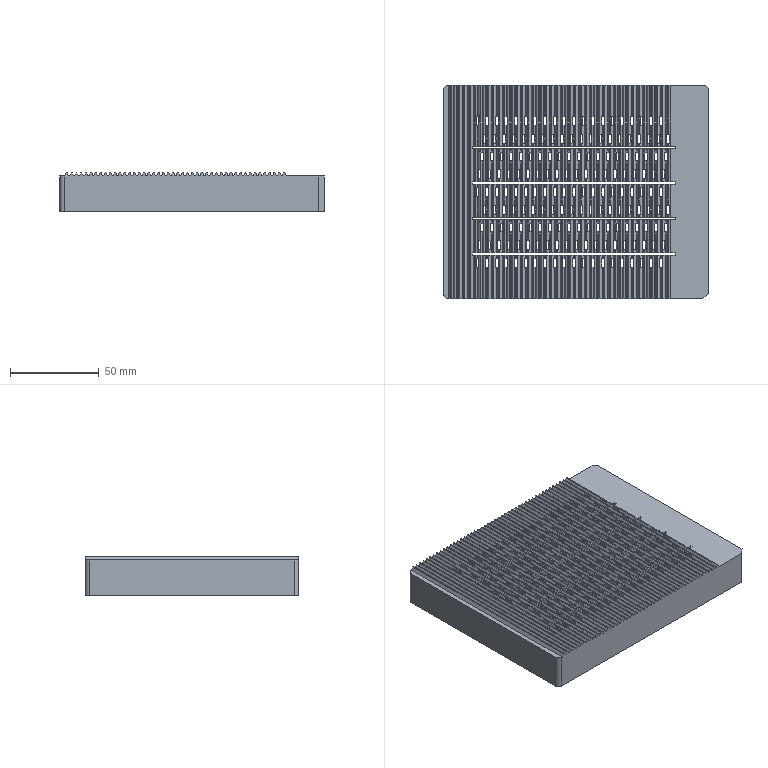Part | STEP file | 1 solid | 1774 faces | box 149 x 120 x 21.74 mm | volume 329380 mm3 | plane 1164 | cylinder 602 | cone 8 | commonest cylinder face diameters 0.8 x305 0.6 x290 5 x7